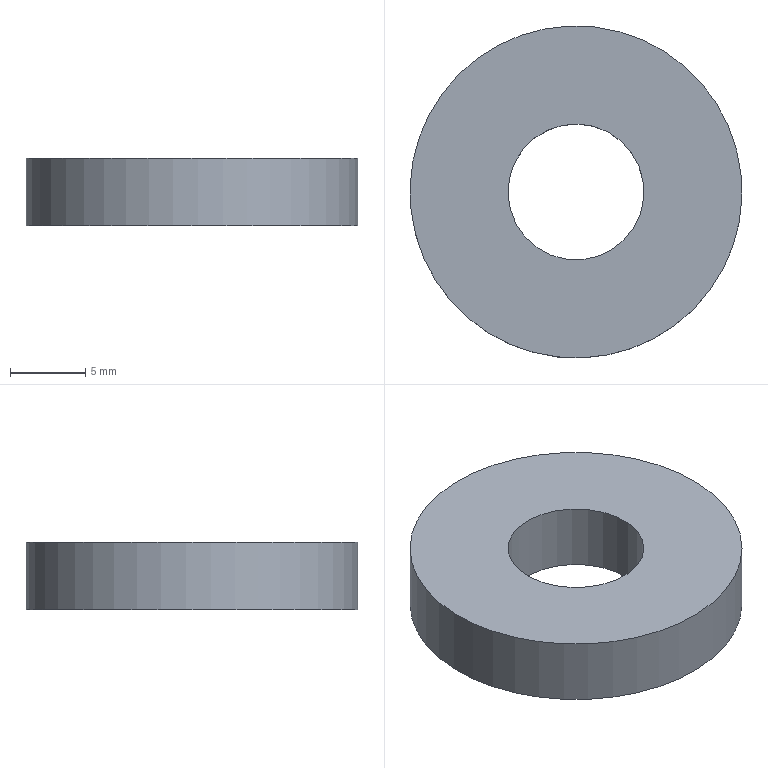Part | NX | features solid 2 | 1 solid | 4 faces | box 22 x 22 x 4.5 mm | volume 1424 mm3 | cylinder 2 | plane 2 | commonest cylinder face diameters 9.007 x1 22 x1
STEP:
#1=CARTESIAN_POINT('',(846.664,160.513,181.129));
#2=VERTEX_POINT('',#1);
#3=CARTESIAN_POINT('',(838.885,168.291,181.129));
#4=DIRECTION('',(0.000000018,-0.000000017,1.));
#5=DIRECTION('',(0.7071,-0.7071,-0.000000025));
#6=AXIS2_PLACEMENT_3D('',#3,#4,#5);
#7=CIRCLE('',#6,11.);
#8=EDGE_CURVE('',#2,#2,#7,.F.);
#9=ORIENTED_EDGE('',*,*,#8,.T.);
#10=EDGE_LOOP('',(#9));
#11=FACE_BOUND('',#10,.T.);
#12=CARTESIAN_POINT('',(846.664,160.513,176.629));
#13=VERTEX_POINT('',#12);
#14=CARTESIAN_POINT('',(838.885,168.291,176.629));
#15=DIRECTION('',(0.000000018,-0.000000017,1.));
#16=DIRECTION('',(0.7071,-0.7071,-0.000000025));
#17=AXIS2_PLACEMENT_3D('',#14,#15,#16);
#18=CIRCLE('',#17,11.);
#19=EDGE_CURVE('',#13,#13,#18,.T.);
#20=ORIENTED_EDGE('',*,*,#19,.T.);
#21=EDGE_LOOP('',(#20));
#22=FACE_BOUND('',#21,.T.);
#23=CARTESIAN_POINT('',(838.885,168.291,181.129));
#24=DIRECTION('',(0.000000018,-0.000000017,1.));
#25=DIRECTION('',(0.9947,-0.1028,-0.00000002));
#26=AXIS2_PLACEMENT_3D('',#23,#24,#25);
#27=CYLINDRICAL_SURFACE('',#26,11.);
#28=ADVANCED_FACE('',(#11,#22),#27,.T.);
#29=CARTESIAN_POINT('',(842.07,165.107,181.129));
#30=VERTEX_POINT('',#29);
#31=CARTESIAN_POINT('',(838.885,168.291,181.129));
#32=DIRECTION('',(0.000000018,-0.000000017,1.));
#33=DIRECTION('',(0.7071,-0.7071,-0.000000025));
#34=AXIS2_PLACEMENT_3D('',#31,#32,#33);
#35=CIRCLE('',#34,4.503);
#36=EDGE_CURVE('',#30,#30,#35,.F.);
#37=ORIENTED_EDGE('',*,*,#36,.T.);
#38=EDGE_LOOP('',(#37));
#39=FACE_BOUND('',#38,.T.);
#40=ORIENTED_EDGE('',*,*,#8,.F.);
#41=EDGE_LOOP('',(#40));
#42=FACE_BOUND('',#41,.T.);
#43=CARTESIAN_POINT('',(844.542,173.948,181.129));
#44=DIRECTION('',(0.000000018,-0.000000017,1.));
#45=DIRECTION('',(-0.7071,-0.7071,0.000000001));
#46=AXIS2_PLACEMENT_3D('',#43,#44,#45);
#47=PLANE('',#46);
#48=ADVANCED_FACE('',(#39,#42),#47,.T.);
#49=ORIENTED_EDGE('',*,*,#36,.F.);
#50=EDGE_LOOP('',(#49));
#51=FACE_BOUND('',#50,.T.);
#52=CARTESIAN_POINT('',(842.07,165.107,176.629));
#53=VERTEX_POINT('',#52);
#54=CARTESIAN_POINT('',(838.885,168.291,176.629));
#55=DIRECTION('',(0.000000018,-0.000000017,1.));
#56=DIRECTION('',(0.7071,-0.7071,-0.000000025));
#57=AXIS2_PLACEMENT_3D('',#54,#55,#56);
#58=CIRCLE('',#57,4.503);
#59=EDGE_CURVE('',#53,#53,#58,.F.);
#60=ORIENTED_EDGE('',*,*,#59,.T.);
#61=EDGE_LOOP('',(#60));
#62=FACE_BOUND('',#61,.T.);
#63=CARTESIAN_POINT('',(838.885,168.291,176.629));
#64=DIRECTION('',(0.000000018,-0.000000017,1.));
#65=DIRECTION('',(-0.7071,-0.7071,0.000000001));
#66=AXIS2_PLACEMENT_3D('',#63,#64,#65);
#67=CYLINDRICAL_SURFACE('',#66,4.503);
#68=ADVANCED_FACE('',(#51,#62),#67,.F.);
#69=ORIENTED_EDGE('',*,*,#19,.F.);
#70=EDGE_LOOP('',(#69));
#71=FACE_BOUND('',#70,.T.);
#72=ORIENTED_EDGE('',*,*,#59,.F.);
#73=EDGE_LOOP('',(#72));
#74=FACE_BOUND('',#73,.T.);
#75=CARTESIAN_POINT('',(844.542,173.948,176.629));
#76=DIRECTION('',(0.000000018,-0.000000017,1.));
#77=DIRECTION('',(-0.7071,-0.7071,0.000000001));
#78=AXIS2_PLACEMENT_3D('',#75,#76,#77);
#79=PLANE('',#78);
#80=ADVANCED_FACE('',(#71,#74),#79,.F.);
#81=CLOSED_SHELL('',(#28,#48,#68,#80));
#82=MANIFOLD_SOLID_BREP('',#81);
#83=(LENGTH_UNIT()NAMED_UNIT(*)SI_UNIT(.MILLI.,.METRE.));
#84=UNCERTAINTY_MEASURE_WITH_UNIT(LENGTH_MEASURE(0.00001),#83,'','');
#85=(NAMED_UNIT(*)PLANE_ANGLE_UNIT()SI_UNIT($,.RADIAN.));
#86=(NAMED_UNIT(*)SI_UNIT($,.STERADIAN.)SOLID_ANGLE_UNIT());
#87=(GEOMETRIC_REPRESENTATION_CONTEXT(3)GLOBAL_UNCERTAINTY_ASSIGNED_CONTEXT((#84))GLOBAL_UNIT_ASSIGNED_CONTEXT((#83,#85,#86))REPRESENTATION_CONTEXT('',''));
#88=ADVANCED_BREP_SHAPE_REPRESENTATION('',(#82),#87);